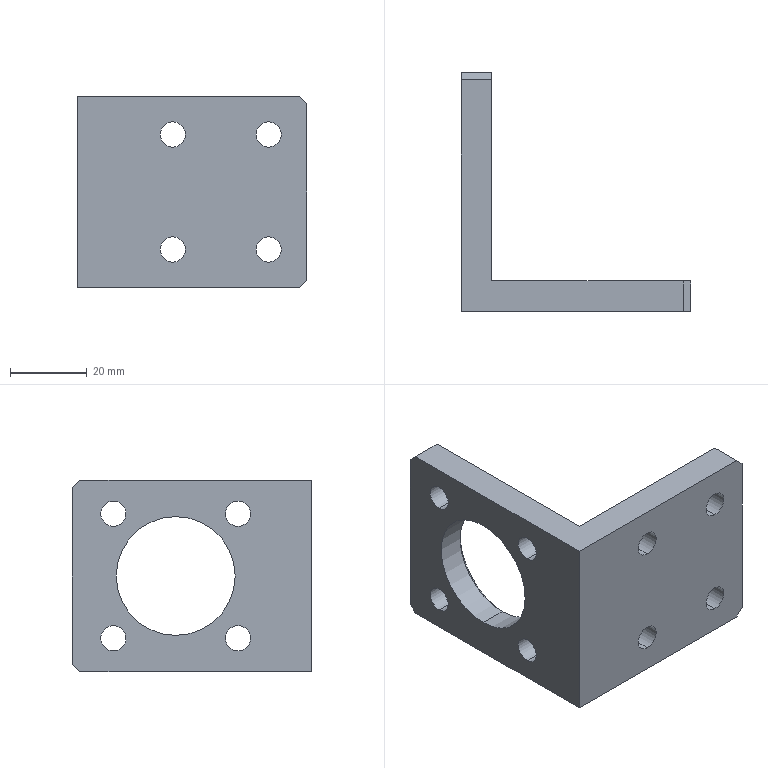Part | SolidWorks | features HoleWzd 3, Chamfer 2, Extrusion 1 | 1 solid | 32 faces | box 60 x 62.5 x 50 mm | volume 37459 mm3 | cylinder 18 | plane 12 | cone 2 | commonest cylinder face diameters 6.6 x16 31 x2
STEP:
#1=CARTESIAN_POINT('',(-15.82,-27.594,36.7));
#2=VERTEX_POINT('',#1);
#3=CARTESIAN_POINT('',(-15.82,-27.594,43.3));
#4=VERTEX_POINT('',#3);
#5=CARTESIAN_POINT('',(-15.82,-27.594,40.));
#6=DIRECTION('',(0.,1.,0.));
#7=DIRECTION('',(0.,0.,1.));
#8=AXIS2_PLACEMENT_3D('',#5,#6,#7);
#9=CIRCLE('',#8,3.3);
#10=EDGE_CURVE('',#2,#4,#9,.T.);
#11=ORIENTED_EDGE('',*,*,#10,.F.);
#12=CARTESIAN_POINT('',(-15.82,-19.594,36.7));
#13=VERTEX_POINT('',#12);
#14=CARTESIAN_POINT('',(-15.82,-19.594,36.7));
#15=DIRECTION('',(0.,1.,0.));
#16=VECTOR('',#15,1000.);
#17=LINE('',#14,#16);
#18=EDGE_CURVE('',#2,#13,#17,.T.);
#19=ORIENTED_EDGE('',*,*,#18,.T.);
#20=CARTESIAN_POINT('',(-15.82,-19.594,43.3));
#21=VERTEX_POINT('',#20);
#22=CARTESIAN_POINT('',(-15.82,-19.594,40.));
#23=DIRECTION('',(0.,1.,0.));
#24=DIRECTION('',(0.,0.,1.));
#25=AXIS2_PLACEMENT_3D('',#22,#23,#24);
#26=CIRCLE('',#25,3.3);
#27=EDGE_CURVE('',#13,#21,#26,.T.);
#28=ORIENTED_EDGE('',*,*,#27,.T.);
#29=CARTESIAN_POINT('',(-15.82,-19.594,43.3));
#30=DIRECTION('',(0.,1.,0.));
#31=VECTOR('',#30,1000.);
#32=LINE('',#29,#31);
#33=EDGE_CURVE('',#4,#21,#32,.T.);
#34=ORIENTED_EDGE('',*,*,#33,.F.);
#35=EDGE_LOOP('',(#11,#19,#28,#34));
#36=FACE_OUTER_BOUND('',#35,.T.);
#37=CARTESIAN_POINT('',(-15.82,-19.594,40.));
#38=DIRECTION('',(0.,1.,0.));
#39=DIRECTION('',(0.,0.,1.));
#40=AXIS2_PLACEMENT_3D('',#37,#38,#39);
#41=CYLINDRICAL_SURFACE('',#40,3.3);
#42=ADVANCED_FACE('',(#36),#41,.F.);
#43=CARTESIAN_POINT('',(-15.82,-27.594,6.7));
#44=VERTEX_POINT('',#43);
#45=CARTESIAN_POINT('',(-15.82,-27.594,13.3));
#46=VERTEX_POINT('',#45);
#47=CARTESIAN_POINT('',(-15.82,-27.594,10.));
#48=DIRECTION('',(0.,1.,0.));
#49=DIRECTION('',(0.,0.,1.));
#50=AXIS2_PLACEMENT_3D('',#47,#48,#49);
#51=CIRCLE('',#50,3.3);
#52=EDGE_CURVE('',#44,#46,#51,.T.);
#53=ORIENTED_EDGE('',*,*,#52,.F.);
#54=CARTESIAN_POINT('',(-15.82,-19.594,6.7));
#55=VERTEX_POINT('',#54);
#56=CARTESIAN_POINT('',(-15.82,-19.594,6.7));
#57=DIRECTION('',(0.,1.,0.));
#58=VECTOR('',#57,1000.);
#59=LINE('',#56,#58);
#60=EDGE_CURVE('',#44,#55,#59,.T.);
#61=ORIENTED_EDGE('',*,*,#60,.T.);
#62=CARTESIAN_POINT('',(-15.82,-19.594,13.3));
#63=VERTEX_POINT('',#62);
#64=CARTESIAN_POINT('',(-15.82,-19.594,10.));
#65=DIRECTION('',(0.,1.,0.));
#66=DIRECTION('',(0.,0.,1.));
#67=AXIS2_PLACEMENT_3D('',#64,#65,#66);
#68=CIRCLE('',#67,3.3);
#69=EDGE_CURVE('',#55,#63,#68,.T.);
#70=ORIENTED_EDGE('',*,*,#69,.T.);
#71=CARTESIAN_POINT('',(-15.82,-19.594,13.3));
#72=DIRECTION('',(0.,1.,0.));
#73=VECTOR('',#72,1000.);
#74=LINE('',#71,#73);
#75=EDGE_CURVE('',#46,#63,#74,.T.);
#76=ORIENTED_EDGE('',*,*,#75,.F.);
#77=EDGE_LOOP('',(#53,#61,#70,#76));
#78=FACE_OUTER_BOUND('',#77,.T.);
#79=CARTESIAN_POINT('',(-15.82,-19.594,10.));
#80=DIRECTION('',(0.,1.,0.));
#81=DIRECTION('',(0.,0.,1.));
#82=AXIS2_PLACEMENT_3D('',#79,#80,#81);
#83=CYLINDRICAL_SURFACE('',#82,3.3);
#84=ADVANCED_FACE('',(#78),#83,.F.);
#85=CARTESIAN_POINT('',(9.18,-27.594,6.7));
#86=VERTEX_POINT('',#85);
#87=CARTESIAN_POINT('',(9.18,-27.594,13.3));
#88=VERTEX_POINT('',#87);
#89=CARTESIAN_POINT('',(9.18,-27.594,10.));
#90=DIRECTION('',(0.,1.,0.));
#91=DIRECTION('',(0.,0.,1.));
#92=AXIS2_PLACEMENT_3D('',#89,#90,#91);
#93=CIRCLE('',#92,3.3);
#94=EDGE_CURVE('',#86,#88,#93,.T.);
#95=ORIENTED_EDGE('',*,*,#94,.F.);
#96=CARTESIAN_POINT('',(9.18,-19.594,6.7));
#97=VERTEX_POINT('',#96);
#98=CARTESIAN_POINT('',(9.18,-19.594,6.7));
#99=DIRECTION('',(0.,1.,0.));
#100=VECTOR('',#99,1000.);
#101=LINE('',#98,#100);
#102=EDGE_CURVE('',#86,#97,#101,.T.);
#103=ORIENTED_EDGE('',*,*,#102,.T.);
#104=CARTESIAN_POINT('',(9.18,-19.594,13.3));
#105=VERTEX_POINT('',#104);
#106=CARTESIAN_POINT('',(9.18,-19.594,10.));
#107=DIRECTION('',(0.,1.,0.));
#108=DIRECTION('',(0.,0.,1.));
#109=AXIS2_PLACEMENT_3D('',#106,#107,#108);
#110=CIRCLE('',#109,3.3);
#111=EDGE_CURVE('',#97,#105,#110,.T.);
#112=ORIENTED_EDGE('',*,*,#111,.T.);
#113=CARTESIAN_POINT('',(9.18,-19.594,13.3));
#114=DIRECTION('',(0.,1.,0.));
#115=VECTOR('',#114,1000.);
#116=LINE('',#113,#115);
#117=EDGE_CURVE('',#88,#105,#116,.T.);
#118=ORIENTED_EDGE('',*,*,#117,.F.);
#119=EDGE_LOOP('',(#95,#103,#112,#118));
#120=FACE_OUTER_BOUND('',#119,.T.);
#121=CARTESIAN_POINT('',(9.18,-19.594,10.));
#122=DIRECTION('',(0.,1.,0.));
#123=DIRECTION('',(0.,0.,1.));
#124=AXIS2_PLACEMENT_3D('',#121,#122,#123);
#125=CYLINDRICAL_SURFACE('',#124,3.3);
#126=ADVANCED_FACE('',(#120),#125,.F.);
#127=CARTESIAN_POINT('',(9.18,-27.594,36.7));
#128=VERTEX_POINT('',#127);
#129=CARTESIAN_POINT('',(9.18,-27.594,43.3));
#130=VERTEX_POINT('',#129);
#131=CARTESIAN_POINT('',(9.18,-27.594,40.));
#132=DIRECTION('',(0.,1.,0.));
#133=DIRECTION('',(0.,0.,1.));
#134=AXIS2_PLACEMENT_3D('',#131,#132,#133);
#135=CIRCLE('',#134,3.3);
#136=EDGE_CURVE('',#128,#130,#135,.T.);
#137=ORIENTED_EDGE('',*,*,#136,.F.);
#138=CARTESIAN_POINT('',(9.18,-19.594,36.7));
#139=VERTEX_POINT('',#138);
#140=CARTESIAN_POINT('',(9.18,-19.594,36.7));
#141=DIRECTION('',(0.,1.,0.));
#142=VECTOR('',#141,1000.);
#143=LINE('',#140,#142);
#144=EDGE_CURVE('',#128,#139,#143,.T.);
#145=ORIENTED_EDGE('',*,*,#144,.T.);
#146=CARTESIAN_POINT('',(9.18,-19.594,43.3));
#147=VERTEX_POINT('',#146);
#148=CARTESIAN_POINT('',(9.18,-19.594,40.));
#149=DIRECTION('',(0.,1.,0.));
#150=DIRECTION('',(0.,0.,1.));
#151=AXIS2_PLACEMENT_3D('',#148,#149,#150);
#152=CIRCLE('',#151,3.3);
#153=EDGE_CURVE('',#139,#147,#152,.T.);
#154=ORIENTED_EDGE('',*,*,#153,.T.);
#155=CARTESIAN_POINT('',(9.18,-19.594,43.3));
#156=DIRECTION('',(0.,1.,0.));
#157=VECTOR('',#156,1000.);
#158=LINE('',#155,#157);
#159=EDGE_CURVE('',#130,#147,#158,.T.);
#160=ORIENTED_EDGE('',*,*,#159,.F.);
#161=EDGE_LOOP('',(#137,#145,#154,#160));
#162=FACE_OUTER_BOUND('',#161,.T.);
#163=CARTESIAN_POINT('',(9.18,-19.594,40.));
#164=DIRECTION('',(0.,1.,0.));
#165=DIRECTION('',(0.,0.,1.));
#166=AXIS2_PLACEMENT_3D('',#163,#164,#165);
#167=CYLINDRICAL_SURFACE('',#166,3.3);
#168=ADVANCED_FACE('',(#162),#167,.F.);
#169=CARTESIAN_POINT('',(-33.82,7.906,40.5));
#170=VERTEX_POINT('',#169);
#171=CARTESIAN_POINT('',(-33.82,7.906,9.5));
#172=VERTEX_POINT('',#171);
#173=CARTESIAN_POINT('',(-33.82,7.906,25.));
#174=DIRECTION('',(1.,0.,0.));
#175=DIRECTION('',(0.,0.,1.));
#176=AXIS2_PLACEMENT_3D('',#173,#174,#175);
#177=CIRCLE('',#176,15.5);
#178=EDGE_CURVE('',#170,#172,#177,.T.);
#179=ORIENTED_EDGE('',*,*,#178,.F.);
#180=CARTESIAN_POINT('',(-32.82,7.906,41.5));
#181=VERTEX_POINT('',#180);
#182=CARTESIAN_POINT('',(-33.82,7.906,40.5));
#183=DIRECTION('',(0.7071,0.,0.7071));
#184=VECTOR('',#183,1000.);
#185=LINE('',#182,#184);
#186=EDGE_CURVE('',#170,#181,#185,.T.);
#187=ORIENTED_EDGE('',*,*,#186,.T.);
#188=CARTESIAN_POINT('',(-32.82,7.906,8.5));
#189=VERTEX_POINT('',#188);
#190=CARTESIAN_POINT('',(-32.82,7.906,25.));
#191=DIRECTION('',(-1.,0.,0.));
#192=DIRECTION('',(0.,0.,1.));
#193=AXIS2_PLACEMENT_3D('',#190,#191,#192);
#194=CIRCLE('',#193,16.5);
#195=EDGE_CURVE('',#189,#181,#194,.T.);
#196=ORIENTED_EDGE('',*,*,#195,.F.);
#197=CARTESIAN_POINT('',(-33.82,7.906,9.5));
#198=DIRECTION('',(0.7071,0.,-0.7071));
#199=VECTOR('',#198,1000.);
#200=LINE('',#197,#199);
#201=EDGE_CURVE('',#172,#189,#200,.T.);
#202=ORIENTED_EDGE('',*,*,#201,.F.);
#203=EDGE_LOOP('',(#179,#187,#196,#202));
#204=FACE_OUTER_BOUND('',#203,.T.);
#205=CARTESIAN_POINT('',(-33.82,7.906,25.));
#206=DIRECTION('',(1.,0.,0.));
#207=DIRECTION('',(0.,0.,-1.));
#208=AXIS2_PLACEMENT_3D('',#205,#206,#207);
#209=CONICAL_SURFACE('',#208,15.5,0.7854);
#210=ADVANCED_FACE('',(#204),#209,.F.);
#211=CARTESIAN_POINT('',(-40.82,7.906,40.5));
#212=VERTEX_POINT('',#211);
#213=CARTESIAN_POINT('',(-40.82,7.906,9.5));
#214=VERTEX_POINT('',#213);
#215=CARTESIAN_POINT('',(-40.82,7.906,25.));
#216=DIRECTION('',(1.,0.,0.));
#217=DIRECTION('',(0.,0.,-1.));
#218=AXIS2_PLACEMENT_3D('',#215,#216,#217);
#219=CIRCLE('',#218,15.5);
#220=EDGE_CURVE('',#212,#214,#219,.T.);
#221=ORIENTED_EDGE('',*,*,#220,.F.);
#222=CARTESIAN_POINT('',(-32.82,7.906,40.5));
#223=DIRECTION('',(1.,0.,0.));
#224=VECTOR('',#223,1000.);
#225=LINE('',#222,#224);
#226=EDGE_CURVE('',#212,#170,#225,.T.);
#227=ORIENTED_EDGE('',*,*,#226,.T.);
#228=ORIENTED_EDGE('',*,*,#178,.T.);
#229=CARTESIAN_POINT('',(-32.82,7.906,9.5));
#230=DIRECTION('',(1.,0.,0.));
#231=VECTOR('',#230,1000.);
#232=LINE('',#229,#231);
#233=EDGE_CURVE('',#214,#172,#232,.T.);
#234=ORIENTED_EDGE('',*,*,#233,.F.);
#235=EDGE_LOOP('',(#221,#227,#228,#234));
#236=FACE_OUTER_BOUND('',#235,.T.);
#237=CARTESIAN_POINT('',(-32.82,7.906,25.));
#238=DIRECTION('',(1.,0.,0.));
#239=DIRECTION('',(0.,0.,-1.));
#240=AXIS2_PLACEMENT_3D('',#237,#238,#239);
#241=CYLINDRICAL_SURFACE('',#240,15.5);
#242=ADVANCED_FACE('',(#236),#241,.F.);
#243=CARTESIAN_POINT('',(-40.82,24.156,44.55));
#244=VERTEX_POINT('',#243);
#245=CARTESIAN_POINT('',(-40.82,24.156,37.95));
#246=VERTEX_POINT('',#245);
#247=CARTESIAN_POINT('',(-40.82,24.156,41.25));
#248=DIRECTION('',(1.,0.,0.));
#249=DIRECTION('',(0.,0.,-1.));
#250=AXIS2_PLACEMENT_3D('',#247,#248,#249);
#251=CIRCLE('',#250,3.3);
#252=EDGE_CURVE('',#244,#246,#251,.T.);
#253=ORIENTED_EDGE('',*,*,#252,.F.);
#254=CARTESIAN_POINT('',(-32.82,24.156,44.55));
#255=VERTEX_POINT('',#254);
#256=CARTESIAN_POINT('',(-32.82,24.156,44.55));
#257=DIRECTION('',(1.,0.,0.));
#258=VECTOR('',#257,1000.);
#259=LINE('',#256,#258);
#260=EDGE_CURVE('',#244,#255,#259,.T.);
#261=ORIENTED_EDGE('',*,*,#260,.T.);
#262=CARTESIAN_POINT('',(-32.82,24.156,37.95));
#263=VERTEX_POINT('',#262);
#264=CARTESIAN_POINT('',(-32.82,24.156,41.25));
#265=DIRECTION('',(1.,0.,0.));
#266=DIRECTION('',(0.,0.,-1.));
#267=AXIS2_PLACEMENT_3D('',#264,#265,#266);
#268=CIRCLE('',#267,3.3);
#269=EDGE_CURVE('',#255,#263,#268,.T.);
#270=ORIENTED_EDGE('',*,*,#269,.T.);
#271=CARTESIAN_POINT('',(-32.82,24.156,37.95));
#272=DIRECTION('',(1.,0.,0.));
#273=VECTOR('',#272,1000.);
#274=LINE('',#271,#273);
#275=EDGE_CURVE('',#246,#263,#274,.T.);
#276=ORIENTED_EDGE('',*,*,#275,.F.);
#277=EDGE_LOOP('',(#253,#261,#270,#276));
#278=FACE_OUTER_BOUND('',#277,.T.);
#279=CARTESIAN_POINT('',(-32.82,24.156,41.25));
#280=DIRECTION('',(1.,0.,0.));
#281=DIRECTION('',(0.,0.,-1.));
#282=AXIS2_PLACEMENT_3D('',#279,#280,#281);
#283=CYLINDRICAL_SURFACE('',#282,3.3);
#284=ADVANCED_FACE('',(#278),#283,.F.);
#285=CARTESIAN_POINT('',(-40.82,24.156,12.05));
#286=VERTEX_POINT('',#285);
#287=CARTESIAN_POINT('',(-40.82,24.156,5.45));
#288=VERTEX_POINT('',#287);
#289=CARTESIAN_POINT('',(-40.82,24.156,8.75));
#290=DIRECTION('',(1.,0.,0.));
#291=DIRECTION('',(0.,0.,-1.));
#292=AXIS2_PLACEMENT_3D('',#289,#290,#291);
#293=CIRCLE('',#292,3.3);
#294=EDGE_CURVE('',#286,#288,#293,.T.);
#295=ORIENTED_EDGE('',*,*,#294,.F.);
#296=CARTESIAN_POINT('',(-32.82,24.156,12.05));
#297=VERTEX_POINT('',#296);
#298=CARTESIAN_POINT('',(-32.82,24.156,12.05));
#299=DIRECTION('',(1.,0.,0.));
#300=VECTOR('',#299,1000.);
#301=LINE('',#298,#300);
#302=EDGE_CURVE('',#286,#297,#301,.T.);
#303=ORIENTED_EDGE('',*,*,#302,.T.);
#304=CARTESIAN_POINT('',(-32.82,24.156,5.45));
#305=VERTEX_POINT('',#304);
#306=CARTESIAN_POINT('',(-32.82,24.156,8.75));
#307=DIRECTION('',(1.,0.,0.));
#308=DIRECTION('',(0.,0.,-1.));
#309=AXIS2_PLACEMENT_3D('',#306,#307,#308);
#310=CIRCLE('',#309,3.3);
#311=EDGE_CURVE('',#297,#305,#310,.T.);
#312=ORIENTED_EDGE('',*,*,#311,.T.);
#313=CARTESIAN_POINT('',(-32.82,24.156,5.45));
#314=DIRECTION('',(1.,0.,0.));
#315=VECTOR('',#314,1000.);
#316=LINE('',#313,#315);
#317=EDGE_CURVE('',#288,#305,#316,.T.);
#318=ORIENTED_EDGE('',*,*,#317,.F.);
#319=EDGE_LOOP('',(#295,#303,#312,#318));
#320=FACE_OUTER_BOUND('',#319,.T.);
#321=CARTESIAN_POINT('',(-32.82,24.156,8.75));
#322=DIRECTION('',(1.,0.,0.));
#323=DIRECTION('',(0.,0.,-1.));
#324=AXIS2_PLACEMENT_3D('',#321,#322,#323);
#325=CYLINDRICAL_SURFACE('',#324,3.3);
#326=ADVANCED_FACE('',(#320),#325,.F.);
#327=CARTESIAN_POINT('',(-40.82,-8.344,12.05));
#328=VERTEX_POINT('',#327);
#329=CARTESIAN_POINT('',(-40.82,-8.344,5.45));
#330=VERTEX_POINT('',#329);
#331=CARTESIAN_POINT('',(-40.82,-8.344,8.75));
#332=DIRECTION('',(1.,0.,0.));
#333=DIRECTION('',(0.,0.,-1.));
#334=AXIS2_PLACEMENT_3D('',#331,#332,#333);
#335=CIRCLE('',#334,3.3);
#336=EDGE_CURVE('',#328,#330,#335,.T.);
#337=ORIENTED_EDGE('',*,*,#336,.F.);
#338=CARTESIAN_POINT('',(-32.82,-8.344,12.05));
#339=VERTEX_POINT('',#338);
#340=CARTESIAN_POINT('',(-32.82,-8.344,12.05));
#341=DIRECTION('',(1.,0.,0.));
#342=VECTOR('',#341,1000.);
#343=LINE('',#340,#342);
#344=EDGE_CURVE('',#328,#339,#343,.T.);
#345=ORIENTED_EDGE('',*,*,#344,.T.);
#346=CARTESIAN_POINT('',(-32.82,-8.344,5.45));
#347=VERTEX_POINT('',#346);
#348=CARTESIAN_POINT('',(-32.82,-8.344,8.75));
#349=DIRECTION('',(1.,0.,0.));
#350=DIRECTION('',(0.,0.,-1.));
#351=AXIS2_PLACEMENT_3D('',#348,#349,#350);
#352=CIRCLE('',#351,3.3);
#353=EDGE_CURVE('',#339,#347,#352,.T.);
#354=ORIENTED_EDGE('',*,*,#353,.T.);
#355=CARTESIAN_POINT('',(-32.82,-8.344,5.45));
#356=DIRECTION('',(1.,0.,0.));
#357=VECTOR('',#356,1000.);
#358=LINE('',#355,#357);
#359=EDGE_CURVE('',#330,#347,#358,.T.);
#360=ORIENTED_EDGE('',*,*,#359,.F.);
#361=EDGE_LOOP('',(#337,#345,#354,#360));
#362=FACE_OUTER_BOUND('',#361,.T.);
#363=CARTESIAN_POINT('',(-32.82,-8.344,8.75));
#364=DIRECTION('',(1.,0.,0.));
#365=DIRECTION('',(0.,0.,-1.));
#366=AXIS2_PLACEMENT_3D('',#363,#364,#365);
#367=CYLINDRICAL_SURFACE('',#366,3.3);
#368=ADVANCED_FACE('',(#362),#367,.F.);
#369=CARTESIAN_POINT('',(-40.82,-8.344,44.55));
#370=VERTEX_POINT('',#369);
#371=CARTESIAN_POINT('',(-40.82,-8.344,37.95));
#372=VERTEX_POINT('',#371);
#373=CARTESIAN_POINT('',(-40.82,-8.344,41.25));
#374=DIRECTION('',(1.,0.,0.));
#375=DIRECTION('',(0.,0.,-1.));
#376=AXIS2_PLACEMENT_3D('',#373,#374,#375);
#377=CIRCLE('',#376,3.3);
#378=EDGE_CURVE('',#370,#372,#377,.T.);
#379=ORIENTED_EDGE('',*,*,#378,.F.);
#380=CARTESIAN_POINT('',(-32.82,-8.344,44.55));
#381=VERTEX_POINT('',#380);
#382=CARTESIAN_POINT('',(-32.82,-8.344,44.55));
#383=DIRECTION('',(1.,0.,0.));
#384=VECTOR('',#383,1000.);
#385=LINE('',#382,#384);
#386=EDGE_CURVE('',#370,#381,#385,.T.);
#387=ORIENTED_EDGE('',*,*,#386,.T.);
#388=CARTESIAN_POINT('',(-32.82,-8.344,37.95));
#389=VERTEX_POINT('',#388);
#390=CARTESIAN_POINT('',(-32.82,-8.344,41.25));
#391=DIRECTION('',(1.,0.,0.));
#392=DIRECTION('',(0.,0.,-1.));
#393=AXIS2_PLACEMENT_3D('',#390,#391,#392);
#394=CIRCLE('',#393,3.3);
#395=EDGE_CURVE('',#381,#389,#394,.T.);
#396=ORIENTED_EDGE('',*,*,#395,.T.);
#397=CARTESIAN_POINT('',(-32.82,-8.344,37.95));
#398=DIRECTION('',(1.,0.,0.));
#399=VECTOR('',#398,1000.);
#400=LINE('',#397,#399);
#401=EDGE_CURVE('',#372,#389,#400,.T.);
#402=ORIENTED_EDGE('',*,*,#401,.F.);
#403=EDGE_LOOP('',(#379,#387,#396,#402));
#404=FACE_OUTER_BOUND('',#403,.T.);
#405=CARTESIAN_POINT('',(-32.82,-8.344,41.25));
#406=DIRECTION('',(1.,0.,0.));
#407=DIRECTION('',(0.,0.,-1.));
#408=AXIS2_PLACEMENT_3D('',#405,#406,#407);
#409=CYLINDRICAL_SURFACE('',#408,3.3);
#410=ADVANCED_FACE('',(#404),#409,.F.);
#411=CARTESIAN_POINT('',(-32.82,34.906,48.));
#412=VERTEX_POINT('',#411);
#413=CARTESIAN_POINT('',(-32.82,34.906,2.));
#414=VERTEX_POINT('',#413);
#415=CARTESIAN_POINT('',(-32.82,34.906,50.));
#416=DIRECTION('',(0.,0.,-1.));
#417=VECTOR('',#416,1000.);
#418=LINE('',#415,#417);
#419=EDGE_CURVE('',#412,#414,#418,.T.);
#420=ORIENTED_EDGE('',*,*,#419,.T.);
#421=CARTESIAN_POINT('',(-40.82,34.906,2.));
#422=VERTEX_POINT('',#421);
#423=CARTESIAN_POINT('',(-32.82,34.906,2.));
#424=DIRECTION('',(-1.,0.,0.));
#425=VECTOR('',#424,1000.);
#426=LINE('',#423,#425);
#427=EDGE_CURVE('',#414,#422,#426,.T.);
#428=ORIENTED_EDGE('',*,*,#427,.T.);
#429=CARTESIAN_POINT('',(-40.82,34.906,48.));
#430=VERTEX_POINT('',#429);
#431=CARTESIAN_POINT('',(-40.82,34.906,50.));
#432=DIRECTION('',(0.,0.,-1.));
#433=VECTOR('',#432,1000.);
#434=LINE('',#431,#433);
#435=EDGE_CURVE('',#430,#422,#434,.T.);
#436=ORIENTED_EDGE('',*,*,#435,.F.);
#437=CARTESIAN_POINT('',(-32.82,34.906,48.));
#438=DIRECTION('',(1.,0.,0.));
#439=VECTOR('',#438,1000.);
#440=LINE('',#437,#439);
#441=EDGE_CURVE('',#430,#412,#440,.T.);
#442=ORIENTED_EDGE('',*,*,#441,.T.);
#443=EDGE_LOOP('',(#420,#428,#436,#442));
#444=FACE_OUTER_BOUND('',#443,.T.);
#445=CARTESIAN_POINT('',(-32.82,34.906,50.));
#446=DIRECTION('',(0.,-1.,0.));
#447=DIRECTION('',(0.,0.,-1.));
#448=AXIS2_PLACEMENT_3D('',#445,#446,#447);
#449=PLANE('',#448);
#450=ADVANCED_FACE('',(#444),#449,.F.);
#451=CARTESIAN_POINT('',(-40.82,7.906,25.));
#452=DIRECTION('',(1.,0.,0.));
#453=DIRECTION('',(0.,0.,-1.));
#454=AXIS2_PLACEMENT_3D('',#451,#452,#453);
#455=CIRCLE('',#454,15.5);
#456=EDGE_CURVE('',#214,#212,#455,.T.);
#457=ORIENTED_EDGE('',*,*,#456,.T.);
#458=ORIENTED_EDGE('',*,*,#220,.T.);
#459=EDGE_LOOP('',(#457,#458));
#460=FACE_BOUND('',#459,.T.);
#461=CARTESIAN_POINT('',(-40.82,24.156,41.25));
#462=DIRECTION('',(1.,0.,0.));
#463=DIRECTION('',(0.,0.,-1.));
#464=AXIS2_PLACEMENT_3D('',#461,#462,#463);
#465=CIRCLE('',#464,3.3);
#466=EDGE_CURVE('',#246,#244,#465,.T.);
#467=ORIENTED_EDGE('',*,*,#466,.T.);
#468=ORIENTED_EDGE('',*,*,#252,.T.);
#469=EDGE_LOOP('',(#467,#468));
#470=FACE_BOUND('',#469,.T.);
#471=CARTESIAN_POINT('',(-40.82,24.156,8.75));
#472=DIRECTION('',(1.,0.,0.));
#473=DIRECTION('',(0.,0.,-1.));
#474=AXIS2_PLACEMENT_3D('',#471,#472,#473);
#475=CIRCLE('',#474,3.3);
#476=EDGE_CURVE('',#288,#286,#475,.T.);
#477=ORIENTED_EDGE('',*,*,#476,.T.);
#478=ORIENTED_EDGE('',*,*,#294,.T.);
#479=EDGE_LOOP('',(#477,#478));
#480=FACE_BOUND('',#479,.T.);
#481=CARTESIAN_POINT('',(-40.82,-8.344,8.75));
#482=DIRECTION('',(1.,0.,0.));
#483=DIRECTION('',(0.,0.,-1.));
#484=AXIS2_PLACEMENT_3D('',#481,#482,#483);
#485=CIRCLE('',#484,3.3);
#486=EDGE_CURVE('',#330,#328,#485,.T.);
#487=ORIENTED_EDGE('',*,*,#486,.T.);
#488=ORIENTED_EDGE('',*,*,#336,.T.);
#489=EDGE_LOOP('',(#487,#488));
#490=FACE_BOUND('',#489,.T.);
#491=CARTESIAN_POINT('',(-40.82,-8.344,41.25));
#492=DIRECTION('',(1.,0.,0.));
#493=DIRECTION('',(0.,0.,-1.));
#494=AXIS2_PLACEMENT_3D('',#491,#492,#493);
#495=CIRCLE('',#494,3.3);
#496=EDGE_CURVE('',#372,#370,#495,.T.);
#497=ORIENTED_EDGE('',*,*,#496,.T.);
#498=ORIENTED_EDGE('',*,*,#378,.T.);
#499=EDGE_LOOP('',(#497,#498));
#500=FACE_BOUND('',#499,.T.);
#501=ORIENTED_EDGE('',*,*,#435,.T.);
#502=CARTESIAN_POINT('',(-40.82,32.906,0.));
#503=VERTEX_POINT('',#502);
#504=CARTESIAN_POINT('',(-40.82,34.906,2.));
#505=DIRECTION('',(0.,-0.7071,-0.7071));
#506=VECTOR('',#505,1000.);
#507=LINE('',#504,#506);
#508=EDGE_CURVE('',#422,#503,#507,.T.);
#509=ORIENTED_EDGE('',*,*,#508,.T.);
#510=CARTESIAN_POINT('',(-40.82,-27.594,0.));
#511=VERTEX_POINT('',#510);
#512=CARTESIAN_POINT('',(-40.82,34.906,0.));
#513=DIRECTION('',(0.,-1.,0.));
#514=VECTOR('',#513,1000.);
#515=LINE('',#512,#514);
#516=EDGE_CURVE('',#503,#511,#515,.T.);
#517=ORIENTED_EDGE('',*,*,#516,.T.);
#518=CARTESIAN_POINT('',(-40.82,-27.594,50.));
#519=VERTEX_POINT('',#518);
#520=CARTESIAN_POINT('',(-40.82,-27.594,50.));
#521=DIRECTION('',(0.,0.,-1.));
#522=VECTOR('',#521,1000.);
#523=LINE('',#520,#522);
#524=EDGE_CURVE('',#519,#511,#523,.T.);
#525=ORIENTED_EDGE('',*,*,#524,.F.);
#526=CARTESIAN_POINT('',(-40.82,32.906,50.));
#527=VERTEX_POINT('',#526);
#528=CARTESIAN_POINT('',(-40.82,34.906,50.));
#529=DIRECTION('',(0.,-1.,0.));
#530=VECTOR('',#529,1000.);
#531=LINE('',#528,#530);
#532=EDGE_CURVE('',#527,#519,#531,.T.);
#533=ORIENTED_EDGE('',*,*,#532,.F.);
#534=CARTESIAN_POINT('',(-40.82,32.906,50.));
#535=DIRECTION('',(0.,0.7071,-0.7071));
#536=VECTOR('',#535,1000.);
#537=LINE('',#534,#536);
#538=EDGE_CURVE('',#527,#430,#537,.T.);
#539=ORIENTED_EDGE('',*,*,#538,.T.);
#540=EDGE_LOOP('',(#501,#509,#517,#525,#533,#539));
#541=FACE_OUTER_BOUND('',#540,.T.);
#542=CARTESIAN_POINT('',(-40.82,34.906,50.));
#543=DIRECTION('',(1.,0.,0.));
#544=DIRECTION('',(0.,1.,0.));
#545=AXIS2_PLACEMENT_3D('',#542,#543,#544);
#546=PLANE('',#545);
#547=ADVANCED_FACE('',(#460,#470,#480,#490,#500,#541),#546,.F.);
#548=CARTESIAN_POINT('',(-15.82,-27.594,40.));
#549=DIRECTION('',(0.,1.,0.));
#550=DIRECTION('',(0.,0.,1.));
#551=AXIS2_PLACEMENT_3D('',#548,#549,#550);
#552=CIRCLE('',#551,3.3);
#553=EDGE_CURVE('',#4,#2,#552,.T.);
#554=ORIENTED_EDGE('',*,*,#553,.T.);
#555=ORIENTED_EDGE('',*,*,#10,.T.);
#556=EDGE_LOOP('',(#554,#555));
#557=FACE_BOUND('',#556,.T.);
#558=CARTESIAN_POINT('',(-15.82,-27.594,10.));
#559=DIRECTION('',(0.,1.,0.));
#560=DIRECTION('',(0.,0.,1.));
#561=AXIS2_PLACEMENT_3D('',#558,#559,#560);
#562=CIRCLE('',#561,3.3);
#563=EDGE_CURVE('',#46,#44,#562,.T.);
#564=ORIENTED_EDGE('',*,*,#563,.T.);
#565=ORIENTED_EDGE('',*,*,#52,.T.);
#566=EDGE_LOOP('',(#564,#565));
#567=FACE_BOUND('',#566,.T.);
#568=CARTESIAN_POINT('',(9.18,-27.594,10.));
#569=DIRECTION('',(0.,1.,0.));
#570=DIRECTION('',(0.,0.,1.));
#571=AXIS2_PLACEMENT_3D('',#568,#569,#570);
#572=CIRCLE('',#571,3.3);
#573=EDGE_CURVE('',#88,#86,#572,.T.);
#574=ORIENTED_EDGE('',*,*,#573,.T.);
#575=ORIENTED_EDGE('',*,*,#94,.T.);
#576=EDGE_LOOP('',(#574,#575));
#577=FACE_BOUND('',#576,.T.);
#578=CARTESIAN_POINT('',(9.18,-27.594,40.));
#579=DIRECTION('',(0.,1.,0.));
#580=DIRECTION('',(0.,0.,1.));
#581=AXIS2_PLACEMENT_3D('',#578,#579,#580);
#582=CIRCLE('',#581,3.3);
#583=EDGE_CURVE('',#130,#128,#582,.T.);
#584=ORIENTED_EDGE('',*,*,#583,.T.);
#585=ORIENTED_EDGE('',*,*,#136,.T.);
#586=EDGE_LOOP('',(#584,#585));
#587=FACE_BOUND('',#586,.T.);
#588=CARTESIAN_POINT('',(17.18,-27.594,0.));
#589=VERTEX_POINT('',#588);
#590=CARTESIAN_POINT('',(-40.82,-27.594,0.));
#591=DIRECTION('',(1.,0.,0.));
#592=VECTOR('',#591,1000.);
#593=LINE('',#590,#592);
#594=EDGE_CURVE('',#511,#589,#593,.T.);
#595=ORIENTED_EDGE('',*,*,#594,.T.);
#596=CARTESIAN_POINT('',(19.18,-27.594,2.));
#597=VERTEX_POINT('',#596);
#598=CARTESIAN_POINT('',(19.18,-27.594,2.));
#599=DIRECTION('',(0.7071,0.,0.7071));
#600=VECTOR('',#599,1000.);
#601=LINE('',#598,#600);
#602=EDGE_CURVE('',#589,#597,#601,.T.);
#603=ORIENTED_EDGE('',*,*,#602,.T.);
#604=CARTESIAN_POINT('',(19.18,-27.594,48.));
#605=VERTEX_POINT('',#604);
#606=CARTESIAN_POINT('',(19.18,-27.594,50.));
#607=DIRECTION('',(0.,0.,-1.));
#608=VECTOR('',#607,1000.);
#609=LINE('',#606,#608);
#610=EDGE_CURVE('',#605,#597,#609,.T.);
#611=ORIENTED_EDGE('',*,*,#610,.F.);
#612=CARTESIAN_POINT('',(17.18,-27.594,50.));
#613=VERTEX_POINT('',#612);
#614=CARTESIAN_POINT('',(17.18,-27.594,50.));
#615=DIRECTION('',(-0.7071,0.,0.7071));
#616=VECTOR('',#615,1000.);
#617=LINE('',#614,#616);
#618=EDGE_CURVE('',#605,#613,#617,.T.);
#619=ORIENTED_EDGE('',*,*,#618,.T.);
#620=CARTESIAN_POINT('',(-40.82,-27.594,50.));
#621=DIRECTION('',(1.,0.,0.));
#622=VECTOR('',#621,1000.);
#623=LINE('',#620,#622);
#624=EDGE_CURVE('',#519,#613,#623,.T.);
#625=ORIENTED_EDGE('',*,*,#624,.F.);
#626=ORIENTED_EDGE('',*,*,#524,.T.);
#627=EDGE_LOOP('',(#595,#603,#611,#619,#625,#626));
#628=FACE_OUTER_BOUND('',#627,.T.);
#629=CARTESIAN_POINT('',(-40.82,-27.594,50.));
#630=DIRECTION('',(0.,1.,0.));
#631=DIRECTION('',(0.,0.,1.));
#632=AXIS2_PLACEMENT_3D('',#629,#630,#631);
#633=PLANE('',#632);
#634=ADVANCED_FACE('',(#557,#567,#577,#587,#628),#633,.F.);
#635=ORIENTED_EDGE('',*,*,#610,.T.);
#636=CARTESIAN_POINT('',(19.18,-19.594,2.));
#637=VERTEX_POINT('',#636);
#638=CARTESIAN_POINT('',(19.18,-27.594,2.));
#639=DIRECTION('',(0.,1.,0.));
#640=VECTOR('',#639,1000.);
#641=LINE('',#638,#640);
#642=EDGE_CURVE('',#597,#637,#641,.T.);
#643=ORIENTED_EDGE('',*,*,#642,.T.);
#644=CARTESIAN_POINT('',(19.18,-19.594,48.));
#645=VERTEX_POINT('',#644);
#646=CARTESIAN_POINT('',(19.18,-19.594,50.));
#647=DIRECTION('',(0.,0.,-1.));
#648=VECTOR('',#647,1000.);
#649=LINE('',#646,#648);
#650=EDGE_CURVE('',#645,#637,#649,.T.);
#651=ORIENTED_EDGE('',*,*,#650,.F.);
#652=CARTESIAN_POINT('',(19.18,-27.594,48.));
#653=DIRECTION('',(0.,-1.,0.));
#654=VECTOR('',#653,1000.);
#655=LINE('',#652,#654);
#656=EDGE_CURVE('',#645,#605,#655,.T.);
#657=ORIENTED_EDGE('',*,*,#656,.T.);
#658=EDGE_LOOP('',(#635,#643,#651,#657));
#659=FACE_OUTER_BOUND('',#658,.T.);
#660=CARTESIAN_POINT('',(19.18,-27.594,50.));
#661=DIRECTION('',(-1.,0.,0.));
#662=DIRECTION('',(0.,0.,1.));
#663=AXIS2_PLACEMENT_3D('',#660,#661,#662);
#664=PLANE('',#663);
#665=ADVANCED_FACE('',(#659),#664,.F.);
#666=CARTESIAN_POINT('',(-15.82,-19.594,40.));
#667=DIRECTION('',(0.,1.,0.));
#668=DIRECTION('',(0.,0.,1.));
#669=AXIS2_PLACEMENT_3D('',#666,#667,#668);
#670=CIRCLE('',#669,3.3);
#671=EDGE_CURVE('',#21,#13,#670,.T.);
#672=ORIENTED_EDGE('',*,*,#671,.F.);
#673=ORIENTED_EDGE('',*,*,#27,.F.);
#674=EDGE_LOOP('',(#672,#673));
#675=FACE_BOUND('',#674,.T.);
#676=CARTESIAN_POINT('',(-15.82,-19.594,10.));
#677=DIRECTION('',(0.,1.,0.));
#678=DIRECTION('',(0.,0.,1.));
#679=AXIS2_PLACEMENT_3D('',#676,#677,#678);
#680=CIRCLE('',#679,3.3);
#681=EDGE_CURVE('',#63,#55,#680,.T.);
#682=ORIENTED_EDGE('',*,*,#681,.F.);
#683=ORIENTED_EDGE('',*,*,#69,.F.);
#684=EDGE_LOOP('',(#682,#683));
#685=FACE_BOUND('',#684,.T.);
#686=CARTESIAN_POINT('',(9.18,-19.594,10.));
#687=DIRECTION('',(0.,1.,0.));
#688=DIRECTION('',(0.,0.,1.));
#689=AXIS2_PLACEMENT_3D('',#686,#687,#688);
#690=CIRCLE('',#689,3.3);
#691=EDGE_CURVE('',#105,#97,#690,.T.);
#692=ORIENTED_EDGE('',*,*,#691,.F.);
#693=ORIENTED_EDGE('',*,*,#111,.F.);
#694=EDGE_LOOP('',(#692,#693));
#695=FACE_BOUND('',#694,.T.);
#696=CARTESIAN_POINT('',(9.18,-19.594,40.));
#697=DIRECTION('',(0.,1.,0.));
#698=DIRECTION('',(0.,0.,1.));
#699=AXIS2_PLACEMENT_3D('',#696,#697,#698);
#700=CIRCLE('',#699,3.3);
#701=EDGE_CURVE('',#147,#139,#700,.T.);
#702=ORIENTED_EDGE('',*,*,#701,.F.);
#703=ORIENTED_EDGE('',*,*,#153,.F.);
#704=EDGE_LOOP('',(#702,#703));
#705=FACE_BOUND('',#704,.T.);
#706=ORIENTED_EDGE('',*,*,#650,.T.);
#707=CARTESIAN_POINT('',(17.18,-19.594,0.));
#708=VERTEX_POINT('',#707);
#709=CARTESIAN_POINT('',(19.18,-19.594,2.));
#710=DIRECTION('',(-0.7071,0.,-0.7071));
#711=VECTOR('',#710,1000.);
#712=LINE('',#709,#711);
#713=EDGE_CURVE('',#637,#708,#712,.T.);
#714=ORIENTED_EDGE('',*,*,#713,.T.);
#715=CARTESIAN_POINT('',(-32.82,-19.594,0.));
#716=VERTEX_POINT('',#715);
#717=CARTESIAN_POINT('',(19.18,-19.594,0.));
#718=DIRECTION('',(-1.,0.,0.));
#719=VECTOR('',#718,1000.);
#720=LINE('',#717,#719);
#721=EDGE_CURVE('',#708,#716,#720,.T.);
#722=ORIENTED_EDGE('',*,*,#721,.T.);
#723=CARTESIAN_POINT('',(-32.82,-19.594,50.));
#724=VERTEX_POINT('',#723);
#725=CARTESIAN_POINT('',(-32.82,-19.594,50.));
#726=DIRECTION('',(0.,0.,-1.));
#727=VECTOR('',#726,1000.);
#728=LINE('',#725,#727);
#729=EDGE_CURVE('',#724,#716,#728,.T.);
#730=ORIENTED_EDGE('',*,*,#729,.F.);
#731=CARTESIAN_POINT('',(17.18,-19.594,50.));
#732=VERTEX_POINT('',#731);
#733=CARTESIAN_POINT('',(19.18,-19.594,50.));
#734=DIRECTION('',(-1.,0.,0.));
#735=VECTOR('',#734,1000.);
#736=LINE('',#733,#735);
#737=EDGE_CURVE('',#732,#724,#736,.T.);
#738=ORIENTED_EDGE('',*,*,#737,.F.);
#739=CARTESIAN_POINT('',(17.18,-19.594,50.));
#740=DIRECTION('',(0.7071,0.,-0.7071));
#741=VECTOR('',#740,1000.);
#742=LINE('',#739,#741);
#743=EDGE_CURVE('',#732,#645,#742,.T.);
#744=ORIENTED_EDGE('',*,*,#743,.T.);
#745=EDGE_LOOP('',(#706,#714,#722,#730,#738,#744));
#746=FACE_OUTER_BOUND('',#745,.T.);
#747=CARTESIAN_POINT('',(19.18,-19.594,50.));
#748=DIRECTION('',(0.,-1.,0.));
#749=DIRECTION('',(0.,0.,-1.));
#750=AXIS2_PLACEMENT_3D('',#747,#748,#749);
#751=PLANE('',#750);
#752=ADVANCED_FACE('',(#675,#685,#695,#705,#746),#751,.F.);
#753=ORIENTED_EDGE('',*,*,#195,.T.);
#754=CARTESIAN_POINT('',(-32.82,7.906,25.));
#755=DIRECTION('',(-1.,0.,0.));
#756=DIRECTION('',(0.,0.,1.));
#757=AXIS2_PLACEMENT_3D('',#754,#755,#756);
#758=CIRCLE('',#757,16.5);
#759=EDGE_CURVE('',#181,#189,#758,.T.);
#760=ORIENTED_EDGE('',*,*,#759,.T.);
#761=EDGE_LOOP('',(#753,#760));
#762=FACE_BOUND('',#761,.T.);
#763=CARTESIAN_POINT('',(-32.82,24.156,41.25));
#764=DIRECTION('',(1.,0.,0.));
#765=DIRECTION('',(0.,0.,-1.));
#766=AXIS2_PLACEMENT_3D('',#763,#764,#765);
#767=CIRCLE('',#766,3.3);
#768=EDGE_CURVE('',#263,#255,#767,.T.);
#769=ORIENTED_EDGE('',*,*,#768,.F.);
#770=ORIENTED_EDGE('',*,*,#269,.F.);
#771=EDGE_LOOP('',(#769,#770));
#772=FACE_BOUND('',#771,.T.);
#773=CARTESIAN_POINT('',(-32.82,24.156,8.75));
#774=DIRECTION('',(1.,0.,0.));
#775=DIRECTION('',(0.,0.,-1.));
#776=AXIS2_PLACEMENT_3D('',#773,#774,#775);
#777=CIRCLE('',#776,3.3);
#778=EDGE_CURVE('',#305,#297,#777,.T.);
#779=ORIENTED_EDGE('',*,*,#778,.F.);
#780=ORIENTED_EDGE('',*,*,#311,.F.);
#781=EDGE_LOOP('',(#779,#780));
#782=FACE_BOUND('',#781,.T.);
#783=CARTESIAN_POINT('',(-32.82,-8.344,8.75));
#784=DIRECTION('',(1.,0.,0.));
#785=DIRECTION('',(0.,0.,-1.));
#786=AXIS2_PLACEMENT_3D('',#783,#784,#785);
#787=CIRCLE('',#786,3.3);
#788=EDGE_CURVE('',#347,#339,#787,.T.);
#789=ORIENTED_EDGE('',*,*,#788,.F.);
#790=ORIENTED_EDGE('',*,*,#353,.F.);
#791=EDGE_LOOP('',(#789,#790));
#792=FACE_BOUND('',#791,.T.);
#793=CARTESIAN_POINT('',(-32.82,-8.344,41.25));
#794=DIRECTION('',(1.,0.,0.));
#795=DIRECTION('',(0.,0.,-1.));
#796=AXIS2_PLACEMENT_3D('',#793,#794,#795);
#797=CIRCLE('',#796,3.3);
#798=EDGE_CURVE('',#389,#381,#797,.T.);
#799=ORIENTED_EDGE('',*,*,#798,.F.);
#800=ORIENTED_EDGE('',*,*,#395,.F.);
#801=EDGE_LOOP('',(#799,#800));
#802=FACE_BOUND('',#801,.T.);
#803=CARTESIAN_POINT('',(-32.82,32.906,0.));
#804=VERTEX_POINT('',#803);
#805=CARTESIAN_POINT('',(-32.82,-19.594,0.));
#806=DIRECTION('',(0.,1.,0.));
#807=VECTOR('',#806,1000.);
#808=LINE('',#805,#807);
#809=EDGE_CURVE('',#716,#804,#808,.T.);
#810=ORIENTED_EDGE('',*,*,#809,.T.);
#811=CARTESIAN_POINT('',(-32.82,34.906,2.));
#812=DIRECTION('',(0.,0.7071,0.7071));
#813=VECTOR('',#812,1000.);
#814=LINE('',#811,#813);
#815=EDGE_CURVE('',#804,#414,#814,.T.);
#816=ORIENTED_EDGE('',*,*,#815,.T.);
#817=ORIENTED_EDGE('',*,*,#419,.F.);
#818=CARTESIAN_POINT('',(-32.82,32.906,50.));
#819=VERTEX_POINT('',#818);
#820=CARTESIAN_POINT('',(-32.82,32.906,50.));
#821=DIRECTION('',(0.,-0.7071,0.7071));
#822=VECTOR('',#821,1000.);
#823=LINE('',#820,#822);
#824=EDGE_CURVE('',#412,#819,#823,.T.);
#825=ORIENTED_EDGE('',*,*,#824,.T.);
#826=CARTESIAN_POINT('',(-32.82,-19.594,50.));
#827=DIRECTION('',(0.,1.,0.));
#828=VECTOR('',#827,1000.);
#829=LINE('',#826,#828);
#830=EDGE_CURVE('',#724,#819,#829,.T.);
#831=ORIENTED_EDGE('',*,*,#830,.F.);
#832=ORIENTED_EDGE('',*,*,#729,.T.);
#833=EDGE_LOOP('',(#810,#816,#817,#825,#831,#832));
#834=FACE_OUTER_BOUND('',#833,.T.);
#835=CARTESIAN_POINT('',(-32.82,-19.594,50.));
#836=DIRECTION('',(-1.,0.,0.));
#837=DIRECTION('',(0.,0.,1.));
#838=AXIS2_PLACEMENT_3D('',#835,#836,#837);
#839=PLANE('',#838);
#840=ADVANCED_FACE('',(#762,#772,#782,#792,#802,#834),#839,.F.);
#841=ORIENTED_EDGE('',*,*,#624,.T.);
#842=CARTESIAN_POINT('',(17.18,-19.594,50.));
#843=DIRECTION('',(0.,1.,0.));
#844=VECTOR('',#843,1000.);
#845=LINE('',#842,#844);
#846=EDGE_CURVE('',#613,#732,#845,.T.);
#847=ORIENTED_EDGE('',*,*,#846,.T.);
#848=ORIENTED_EDGE('',*,*,#737,.T.);
#849=ORIENTED_EDGE('',*,*,#830,.T.);
#850=CARTESIAN_POINT('',(-40.82,32.906,50.));
#851=DIRECTION('',(-1.,0.,0.));
#852=VECTOR('',#851,1000.);
#853=LINE('',#850,#852);
#854=EDGE_CURVE('',#819,#527,#853,.T.);
#855=ORIENTED_EDGE('',*,*,#854,.T.);
#856=ORIENTED_EDGE('',*,*,#532,.T.);
#857=EDGE_LOOP('',(#841,#847,#848,#849,#855,#856));
#858=FACE_OUTER_BOUND('',#857,.T.);
#859=CARTESIAN_POINT('',(0.,0.,50.));
#860=DIRECTION('',(0.,0.,1.));
#861=DIRECTION('',(1.,0.,0.));
#862=AXIS2_PLACEMENT_3D('',#859,#860,#861);
#863=PLANE('',#862);
#864=ADVANCED_FACE('',(#858),#863,.T.);
#865=ORIENTED_EDGE('',*,*,#721,.F.);
#866=CARTESIAN_POINT('',(17.18,0.,0.));
#867=DIRECTION('',(0.,-1.,0.));
#868=VECTOR('',#867,1000.);
#869=LINE('',#866,#868);
#870=EDGE_CURVE('',#708,#589,#869,.T.);
#871=ORIENTED_EDGE('',*,*,#870,.T.);
#872=ORIENTED_EDGE('',*,*,#594,.F.);
#873=ORIENTED_EDGE('',*,*,#516,.F.);
#874=CARTESIAN_POINT('',(0.,32.906,0.));
#875=DIRECTION('',(1.,0.,0.));
#876=VECTOR('',#875,1000.);
#877=LINE('',#874,#876);
#878=EDGE_CURVE('',#503,#804,#877,.T.);
#879=ORIENTED_EDGE('',*,*,#878,.T.);
#880=ORIENTED_EDGE('',*,*,#809,.F.);
#881=EDGE_LOOP('',(#865,#871,#872,#873,#879,#880));
#882=FACE_OUTER_BOUND('',#881,.T.);
#883=CARTESIAN_POINT('',(0.,0.,0.));
#884=DIRECTION('',(0.,0.,1.));
#885=DIRECTION('',(1.,0.,0.));
#886=AXIS2_PLACEMENT_3D('',#883,#884,#885);
#887=PLANE('',#886);
#888=ADVANCED_FACE('',(#882),#887,.F.);
#889=ORIENTED_EDGE('',*,*,#386,.F.);
#890=ORIENTED_EDGE('',*,*,#496,.F.);
#891=ORIENTED_EDGE('',*,*,#401,.T.);
#892=ORIENTED_EDGE('',*,*,#798,.T.);
#893=EDGE_LOOP('',(#889,#890,#891,#892));
#894=FACE_OUTER_BOUND('',#893,.T.);
#895=CARTESIAN_POINT('',(-32.82,-8.344,41.25));
#896=DIRECTION('',(1.,0.,0.));
#897=DIRECTION('',(0.,0.,-1.));
#898=AXIS2_PLACEMENT_3D('',#895,#896,#897);
#899=CYLINDRICAL_SURFACE('',#898,3.3);
#900=ADVANCED_FACE('',(#894),#899,.F.);
#901=ORIENTED_EDGE('',*,*,#344,.F.);
#902=ORIENTED_EDGE('',*,*,#486,.F.);
#903=ORIENTED_EDGE('',*,*,#359,.T.);
#904=ORIENTED_EDGE('',*,*,#788,.T.);
#905=EDGE_LOOP('',(#901,#902,#903,#904));
#906=FACE_OUTER_BOUND('',#905,.T.);
#907=CARTESIAN_POINT('',(-32.82,-8.344,8.75));
#908=DIRECTION('',(1.,0.,0.));
#909=DIRECTION('',(0.,0.,-1.));
#910=AXIS2_PLACEMENT_3D('',#907,#908,#909);
#911=CYLINDRICAL_SURFACE('',#910,3.3);
#912=ADVANCED_FACE('',(#906),#911,.F.);
#913=ORIENTED_EDGE('',*,*,#302,.F.);
#914=ORIENTED_EDGE('',*,*,#476,.F.);
#915=ORIENTED_EDGE('',*,*,#317,.T.);
#916=ORIENTED_EDGE('',*,*,#778,.T.);
#917=EDGE_LOOP('',(#913,#914,#915,#916));
#918=FACE_OUTER_BOUND('',#917,.T.);
#919=CARTESIAN_POINT('',(-32.82,24.156,8.75));
#920=DIRECTION('',(1.,0.,0.));
#921=DIRECTION('',(0.,0.,-1.));
#922=AXIS2_PLACEMENT_3D('',#919,#920,#921);
#923=CYLINDRICAL_SURFACE('',#922,3.3);
#924=ADVANCED_FACE('',(#918),#923,.F.);
#925=ORIENTED_EDGE('',*,*,#260,.F.);
#926=ORIENTED_EDGE('',*,*,#466,.F.);
#927=ORIENTED_EDGE('',*,*,#275,.T.);
#928=ORIENTED_EDGE('',*,*,#768,.T.);
#929=EDGE_LOOP('',(#925,#926,#927,#928));
#930=FACE_OUTER_BOUND('',#929,.T.);
#931=CARTESIAN_POINT('',(-32.82,24.156,41.25));
#932=DIRECTION('',(1.,0.,0.));
#933=DIRECTION('',(0.,0.,-1.));
#934=AXIS2_PLACEMENT_3D('',#931,#932,#933);
#935=CYLINDRICAL_SURFACE('',#934,3.3);
#936=ADVANCED_FACE('',(#930),#935,.F.);
#937=ORIENTED_EDGE('',*,*,#226,.F.);
#938=ORIENTED_EDGE('',*,*,#456,.F.);
#939=ORIENTED_EDGE('',*,*,#233,.T.);
#940=CARTESIAN_POINT('',(-33.82,7.906,25.));
#941=DIRECTION('',(1.,0.,0.));
#942=DIRECTION('',(0.,0.,1.));
#943=AXIS2_PLACEMENT_3D('',#940,#941,#942);
#944=CIRCLE('',#943,15.5);
#945=EDGE_CURVE('',#172,#170,#944,.T.);
#946=ORIENTED_EDGE('',*,*,#945,.T.);
#947=EDGE_LOOP('',(#937,#938,#939,#946));
#948=FACE_OUTER_BOUND('',#947,.T.);
#949=CARTESIAN_POINT('',(-32.82,7.906,25.));
#950=DIRECTION('',(1.,0.,0.));
#951=DIRECTION('',(0.,0.,-1.));
#952=AXIS2_PLACEMENT_3D('',#949,#950,#951);
#953=CYLINDRICAL_SURFACE('',#952,15.5);
#954=ADVANCED_FACE('',(#948),#953,.F.);
#955=ORIENTED_EDGE('',*,*,#186,.F.);
#956=ORIENTED_EDGE('',*,*,#945,.F.);
#957=ORIENTED_EDGE('',*,*,#201,.T.);
#958=ORIENTED_EDGE('',*,*,#759,.F.);
#959=EDGE_LOOP('',(#955,#956,#957,#958));
#960=FACE_OUTER_BOUND('',#959,.T.);
#961=CARTESIAN_POINT('',(-33.82,7.906,25.));
#962=DIRECTION('',(1.,0.,0.));
#963=DIRECTION('',(0.,0.,-1.));
#964=AXIS2_PLACEMENT_3D('',#961,#962,#963);
#965=CONICAL_SURFACE('',#964,15.5,0.7854);
#966=ADVANCED_FACE('',(#960),#965,.F.);
#967=ORIENTED_EDGE('',*,*,#602,.F.);
#968=ORIENTED_EDGE('',*,*,#870,.F.);
#969=ORIENTED_EDGE('',*,*,#713,.F.);
#970=ORIENTED_EDGE('',*,*,#642,.F.);
#971=EDGE_LOOP('',(#967,#968,#969,#970));
#972=FACE_OUTER_BOUND('',#971,.T.);
#973=CARTESIAN_POINT('',(19.18,-27.594,2.));
#974=DIRECTION('',(-0.7071,0.,0.7071));
#975=DIRECTION('',(0.,1.,0.));
#976=AXIS2_PLACEMENT_3D('',#973,#974,#975);
#977=PLANE('',#976);
#978=ADVANCED_FACE('',(#972),#977,.F.);
#979=ORIENTED_EDGE('',*,*,#618,.F.);
#980=ORIENTED_EDGE('',*,*,#656,.F.);
#981=ORIENTED_EDGE('',*,*,#743,.F.);
#982=ORIENTED_EDGE('',*,*,#846,.F.);
#983=EDGE_LOOP('',(#979,#980,#981,#982));
#984=FACE_OUTER_BOUND('',#983,.T.);
#985=CARTESIAN_POINT('',(17.18,0.,50.));
#986=DIRECTION('',(0.7071,0.,0.7071));
#987=DIRECTION('',(0.,-1.,0.));
#988=AXIS2_PLACEMENT_3D('',#985,#986,#987);
#989=PLANE('',#988);
#990=ADVANCED_FACE('',(#984),#989,.T.);
#991=ORIENTED_EDGE('',*,*,#815,.F.);
#992=ORIENTED_EDGE('',*,*,#878,.F.);
#993=ORIENTED_EDGE('',*,*,#508,.F.);
#994=ORIENTED_EDGE('',*,*,#427,.F.);
#995=EDGE_LOOP('',(#991,#992,#993,#994));
#996=FACE_OUTER_BOUND('',#995,.T.);
#997=CARTESIAN_POINT('',(-32.82,34.906,2.));
#998=DIRECTION('',(0.,-0.7071,0.7071));
#999=DIRECTION('',(-1.,0.,0.));
#1000=AXIS2_PLACEMENT_3D('',#997,#998,#999);
#1001=PLANE('',#1000);
#1002=ADVANCED_FACE('',(#996),#1001,.F.);
#1003=ORIENTED_EDGE('',*,*,#824,.F.);
#1004=ORIENTED_EDGE('',*,*,#441,.F.);
#1005=ORIENTED_EDGE('',*,*,#538,.F.);
#1006=ORIENTED_EDGE('',*,*,#854,.F.);
#1007=EDGE_LOOP('',(#1003,#1004,#1005,#1006));
#1008=FACE_OUTER_BOUND('',#1007,.T.);
#1009=CARTESIAN_POINT('',(0.,32.906,50.));
#1010=DIRECTION('',(0.,0.7071,0.7071));
#1011=DIRECTION('',(1.,0.,0.));
#1012=AXIS2_PLACEMENT_3D('',#1009,#1010,#1011);
#1013=PLANE('',#1012);
#1014=ADVANCED_FACE('',(#1008),#1013,.T.);
#1015=ORIENTED_EDGE('',*,*,#144,.F.);
#1016=ORIENTED_EDGE('',*,*,#583,.F.);
#1017=ORIENTED_EDGE('',*,*,#159,.T.);
#1018=ORIENTED_EDGE('',*,*,#701,.T.);
#1019=EDGE_LOOP('',(#1015,#1016,#1017,#1018));
#1020=FACE_OUTER_BOUND('',#1019,.T.);
#1021=CARTESIAN_POINT('',(9.18,-19.594,40.));
#1022=DIRECTION('',(0.,1.,0.));
#1023=DIRECTION('',(0.,0.,1.));
#1024=AXIS2_PLACEMENT_3D('',#1021,#1022,#1023);
#1025=CYLINDRICAL_SURFACE('',#1024,3.3);
#1026=ADVANCED_FACE('',(#1020),#1025,.F.);
#1027=ORIENTED_EDGE('',*,*,#102,.F.);
#1028=ORIENTED_EDGE('',*,*,#573,.F.);
#1029=ORIENTED_EDGE('',*,*,#117,.T.);
#1030=ORIENTED_EDGE('',*,*,#691,.T.);
#1031=EDGE_LOOP('',(#1027,#1028,#1029,#1030));
#1032=FACE_OUTER_BOUND('',#1031,.T.);
#1033=CARTESIAN_POINT('',(9.18,-19.594,10.));
#1034=DIRECTION('',(0.,1.,0.));
#1035=DIRECTION('',(0.,0.,1.));
#1036=AXIS2_PLACEMENT_3D('',#1033,#1034,#1035);
#1037=CYLINDRICAL_SURFACE('',#1036,3.3);
#1038=ADVANCED_FACE('',(#1032),#1037,.F.);
#1039=ORIENTED_EDGE('',*,*,#60,.F.);
#1040=ORIENTED_EDGE('',*,*,#563,.F.);
#1041=ORIENTED_EDGE('',*,*,#75,.T.);
#1042=ORIENTED_EDGE('',*,*,#681,.T.);
#1043=EDGE_LOOP('',(#1039,#1040,#1041,#1042));
#1044=FACE_OUTER_BOUND('',#1043,.T.);
#1045=CARTESIAN_POINT('',(-15.82,-19.594,10.));
#1046=DIRECTION('',(0.,1.,0.));
#1047=DIRECTION('',(0.,0.,1.));
#1048=AXIS2_PLACEMENT_3D('',#1045,#1046,#1047);
#1049=CYLINDRICAL_SURFACE('',#1048,3.3);
#1050=ADVANCED_FACE('',(#1044),#1049,.F.);
#1051=ORIENTED_EDGE('',*,*,#18,.F.);
#1052=ORIENTED_EDGE('',*,*,#553,.F.);
#1053=ORIENTED_EDGE('',*,*,#33,.T.);
#1054=ORIENTED_EDGE('',*,*,#671,.T.);
#1055=EDGE_LOOP('',(#1051,#1052,#1053,#1054));
#1056=FACE_OUTER_BOUND('',#1055,.T.);
#1057=CARTESIAN_POINT('',(-15.82,-19.594,40.));
#1058=DIRECTION('',(0.,1.,0.));
#1059=DIRECTION('',(0.,0.,1.));
#1060=AXIS2_PLACEMENT_3D('',#1057,#1058,#1059);
#1061=CYLINDRICAL_SURFACE('',#1060,3.3);
#1062=ADVANCED_FACE('',(#1056),#1061,.F.);
#1063=CLOSED_SHELL('',(#42,#84,#126,#168,#210,#242,#284,#326,#368,#410,#450,#547,#634,#665,#752,#840,#864,#888,#900,#912,#924,#936,#954,#966,#978,#990,#1002,#1014,#1026,#1038,#1050,#1062));
#1064=MANIFOLD_SOLID_BREP('',#1063);
#1065=CARTESIAN_POINT('',(0.,0.,0.));
#1066=DIRECTION('',(0.,0.,1.));
#1067=DIRECTION('',(1.,0.,0.));
#1068=AXIS2_PLACEMENT_3D('',#1065,#1066,#1067);
#1069=(LENGTH_UNIT()NAMED_UNIT(*)SI_UNIT(.MILLI.,.METRE.));
#1070=UNCERTAINTY_MEASURE_WITH_UNIT(LENGTH_MEASURE(0.00001),#1069,'','');
#1071=(NAMED_UNIT(*)PLANE_ANGLE_UNIT()SI_UNIT($,.RADIAN.));
#1072=(NAMED_UNIT(*)SI_UNIT($,.STERADIAN.)SOLID_ANGLE_UNIT());
#1073=(GEOMETRIC_REPRESENTATION_CONTEXT(3)GLOBAL_UNCERTAINTY_ASSIGNED_CONTEXT((#1070))GLOBAL_UNIT_ASSIGNED_CONTEXT((#1069,#1071,#1072))REPRESENTATION_CONTEXT('',''));
#1074=ADVANCED_BREP_SHAPE_REPRESENTATION('',(#1064,#1068),#1073);